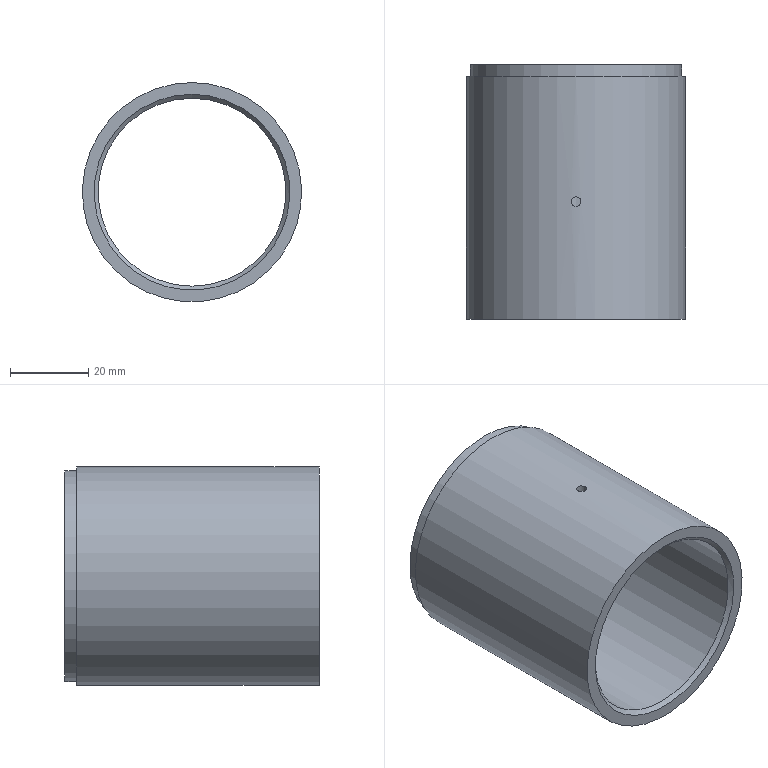Part | STEP file | JBJ-P-1016-01 | 1 solid | 8 faces | box 56 x 65 x 56 mm | volume 41860 mm3 | cylinder 4 | plane 3 | cone 1 | commonest cylinder face diameters 2.5 x1 48 x1 54 x1 56 x1
STEP:
#1=CARTESIAN_POINT('',(0.,62.,27.));
#2=VERTEX_POINT('',#1);
#3=CARTESIAN_POINT('',(0.,62.,0.));
#4=DIRECTION('',(0.,1.,0.));
#5=DIRECTION('',(0.,0.,1.));
#6=AXIS2_PLACEMENT_3D('',#3,#4,#5);
#7=CIRCLE('',#6,27.);
#8=EDGE_CURVE('',#2,#2,#7,.T.);
#9=ORIENTED_EDGE('',*,*,#8,.F.);
#10=EDGE_LOOP('',(#9));
#11=FACE_BOUND('',#10,.T.);
#12=CARTESIAN_POINT('',(0.,62.,28.));
#13=VERTEX_POINT('',#12);
#14=CARTESIAN_POINT('',(0.,62.,0.));
#15=DIRECTION('',(0.,1.,0.));
#16=DIRECTION('',(0.,0.,1.));
#17=AXIS2_PLACEMENT_3D('',#14,#15,#16);
#18=CIRCLE('',#17,28.);
#19=EDGE_CURVE('',#13,#13,#18,.T.);
#20=ORIENTED_EDGE('',*,*,#19,.T.);
#21=EDGE_LOOP('',(#20));
#22=FACE_OUTER_BOUND('',#21,.T.);
#23=CARTESIAN_POINT('',(0.,62.,0.));
#24=DIRECTION('',(0.,1.,0.));
#25=DIRECTION('',(0.,0.,1.));
#26=AXIS2_PLACEMENT_3D('',#23,#24,#25);
#27=PLANE('',#26);
#28=ADVANCED_FACE('',(#11,#22),#27,.T.);
#29=CARTESIAN_POINT('',(0.,0.,25.));
#30=VERTEX_POINT('',#29);
#31=CARTESIAN_POINT('',(0.,0.,0.));
#32=DIRECTION('',(0.,1.,0.));
#33=DIRECTION('',(0.,0.,1.));
#34=AXIS2_PLACEMENT_3D('',#31,#32,#33);
#35=CIRCLE('',#34,25.);
#36=EDGE_CURVE('',#30,#30,#35,.T.);
#37=ORIENTED_EDGE('',*,*,#36,.T.);
#38=EDGE_LOOP('',(#37));
#39=FACE_BOUND('',#38,.T.);
#40=CARTESIAN_POINT('',(0.,0.,28.));
#41=VERTEX_POINT('',#40);
#42=CARTESIAN_POINT('',(0.,0.,0.));
#43=DIRECTION('',(0.,1.,0.));
#44=DIRECTION('',(0.,0.,1.));
#45=AXIS2_PLACEMENT_3D('',#42,#43,#44);
#46=CIRCLE('',#45,28.);
#47=EDGE_CURVE('',#41,#41,#46,.T.);
#48=ORIENTED_EDGE('',*,*,#47,.F.);
#49=EDGE_LOOP('',(#48));
#50=FACE_OUTER_BOUND('',#49,.T.);
#51=CARTESIAN_POINT('',(0.,0.,0.));
#52=DIRECTION('',(0.,1.,0.));
#53=DIRECTION('',(0.,0.,1.));
#54=AXIS2_PLACEMENT_3D('',#51,#52,#53);
#55=PLANE('',#54);
#56=ADVANCED_FACE('',(#39,#50),#55,.F.);
#57=CARTESIAN_POINT('',(0.,28.75,28.));
#58=VERTEX_POINT('',#57);
#59=CARTESIAN_POINT('',(0.,28.75,28.));
#60=CARTESIAN_POINT('',(-0.1652,28.75,28.));
#61=CARTESIAN_POINT('',(-0.3273,28.783,27.998));
#62=CARTESIAN_POINT('',(-0.63,28.908,27.993));
#63=CARTESIAN_POINT('',(-0.7687,29.001,27.99));
#64=CARTESIAN_POINT('',(-0.9993,29.232,27.982));
#65=CARTESIAN_POINT('',(-1.092,29.371,27.979));
#66=CARTESIAN_POINT('',(-1.217,29.672,27.974));
#67=CARTESIAN_POINT('',(-1.25,29.836,27.972));
#68=CARTESIAN_POINT('',(-1.25,30.162,27.972));
#69=CARTESIAN_POINT('',(-1.218,30.326,27.974));
#70=CARTESIAN_POINT('',(-1.093,30.629,27.979));
#71=CARTESIAN_POINT('',(-1.001,30.767,27.982));
#72=CARTESIAN_POINT('',(-0.7677,31.,27.99));
#73=CARTESIAN_POINT('',(-0.6301,31.092,27.993));
#74=CARTESIAN_POINT('',(-0.4029,31.186,27.997));
#75=CARTESIAN_POINT('',(-0.325,31.21,27.998));
#76=CARTESIAN_POINT('',(-0.1649,31.242,28.));
#77=CARTESIAN_POINT('',(-0.08202,31.25,28.));
#78=CARTESIAN_POINT('',(0.1627,31.25,28.));
#79=CARTESIAN_POINT('',(0.3272,31.217,27.998));
#80=CARTESIAN_POINT('',(0.6281,31.093,27.993));
#81=CARTESIAN_POINT('',(0.7677,31.,27.99));
#82=CARTESIAN_POINT('',(0.9984,30.77,27.982));
#83=CARTESIAN_POINT('',(1.091,30.631,27.979));
#84=CARTESIAN_POINT('',(1.217,30.329,27.974));
#85=CARTESIAN_POINT('',(1.25,30.166,27.972));
#86=CARTESIAN_POINT('',(1.25,29.836,27.972));
#87=CARTESIAN_POINT('',(1.218,29.674,27.974));
#88=CARTESIAN_POINT('',(1.124,29.447,27.977));
#89=CARTESIAN_POINT('',(1.085,29.375,27.979));
#90=CARTESIAN_POINT('',(0.995,29.239,27.982));
#91=CARTESIAN_POINT('',(0.9422,29.175,27.984));
#92=CARTESIAN_POINT('',(0.7693,29.001,27.99));
#93=CARTESIAN_POINT('',(0.63,28.908,27.993));
#94=CARTESIAN_POINT('',(0.3293,28.783,27.998));
#95=CARTESIAN_POINT('',(0.1652,28.75,28.));
#96=CARTESIAN_POINT('',(0.,28.75,28.));
#97=B_SPLINE_CURVE_WITH_KNOTS('',3,(#59,#60,#61,#62,#63,#64,#65,#66,#67,#68,#69,#70,#71,#72,#73,#74,#75,#76,#77,#78,#79,#80,#81,#82,#83,#84,#85,#86,#87,#88,#89,#90,#91,#92,#93,#94,#95,#96),.UNSPECIFIED.,.T.,.F.,(4,2,2,2,2,2,2,2,2,2,2,2,2,2,2,2,2,2,4),(0.,0.0004885,0.000977,0.001466,0.001954,0.002443,0.002931,0.00342,0.003664,0.003908,0.004397,0.004885,0.005374,0.005862,0.006351,0.006595,0.006839,0.007328,0.007816),.UNSPECIFIED.);
#98=EDGE_CURVE('',#58,#58,#97,.T.);
#99=ORIENTED_EDGE('',*,*,#98,.T.);
#100=EDGE_LOOP('',(#99));
#101=FACE_BOUND('',#100,.T.);
#102=ORIENTED_EDGE('',*,*,#19,.F.);
#103=EDGE_LOOP('',(#102));
#104=FACE_OUTER_BOUND('',#103,.T.);
#105=ORIENTED_EDGE('',*,*,#47,.T.);
#106=EDGE_LOOP('',(#105));
#107=FACE_OUTER_BOUND('',#106,.T.);
#108=CARTESIAN_POINT('',(0.,62.,0.));
#109=DIRECTION('',(0.,-1.,0.));
#110=DIRECTION('',(0.,0.,-1.));
#111=AXIS2_PLACEMENT_3D('',#108,#109,#110);
#112=CYLINDRICAL_SURFACE('',#111,28.);
#113=ADVANCED_FACE('',(#101,#104,#107),#112,.T.);
#114=CARTESIAN_POINT('',(0.,1.,24.));
#115=VERTEX_POINT('',#114);
#116=CARTESIAN_POINT('',(0.,1.,0.));
#117=DIRECTION('',(0.,-1.,0.));
#118=DIRECTION('',(0.,0.,1.));
#119=AXIS2_PLACEMENT_3D('',#116,#117,#118);
#120=CIRCLE('',#119,24.);
#121=EDGE_CURVE('',#115,#115,#120,.T.);
#122=ORIENTED_EDGE('',*,*,#121,.T.);
#123=EDGE_LOOP('',(#122));
#124=FACE_OUTER_BOUND('',#123,.T.);
#125=CARTESIAN_POINT('',(-1.25,30.,23.967));
#126=VERTEX_POINT('',#125);
#127=CARTESIAN_POINT('',(-1.25,30.,23.967));
#128=CARTESIAN_POINT('',(-1.25,30.165,23.967));
#129=CARTESIAN_POINT('',(-1.217,30.327,23.969));
#130=CARTESIAN_POINT('',(-1.092,30.63,23.975));
#131=CARTESIAN_POINT('',(-0.9991,30.769,23.979));
#132=CARTESIAN_POINT('',(-0.7685,30.999,23.988));
#133=CARTESIAN_POINT('',(-0.6291,31.092,23.992));
#134=CARTESIAN_POINT('',(-0.3282,31.217,23.998));
#135=CARTESIAN_POINT('',(-0.1637,31.25,24.));
#136=CARTESIAN_POINT('',(0.1624,31.25,24.));
#137=CARTESIAN_POINT('',(0.3263,31.218,23.998));
#138=CARTESIAN_POINT('',(0.629,31.093,23.992));
#139=CARTESIAN_POINT('',(0.7667,31.001,23.988));
#140=CARTESIAN_POINT('',(1.,30.768,23.979));
#141=CARTESIAN_POINT('',(1.092,30.63,23.975));
#142=CARTESIAN_POINT('',(1.186,30.403,23.971));
#143=CARTESIAN_POINT('',(1.21,30.325,23.969));
#144=CARTESIAN_POINT('',(1.242,30.165,23.968));
#145=CARTESIAN_POINT('',(1.25,30.082,23.967));
#146=CARTESIAN_POINT('',(1.25,29.837,23.967));
#147=CARTESIAN_POINT('',(1.217,29.673,23.969));
#148=CARTESIAN_POINT('',(1.093,29.372,23.975));
#149=CARTESIAN_POINT('',(0.9999,29.232,23.979));
#150=CARTESIAN_POINT('',(0.7696,29.002,23.988));
#151=CARTESIAN_POINT('',(0.6309,28.909,23.992));
#152=CARTESIAN_POINT('',(0.3286,28.783,23.998));
#153=CARTESIAN_POINT('',(0.1662,28.75,24.));
#154=CARTESIAN_POINT('',(-0.1637,28.75,24.));
#155=CARTESIAN_POINT('',(-0.326,28.782,23.998));
#156=CARTESIAN_POINT('',(-0.5534,28.876,23.994));
#157=CARTESIAN_POINT('',(-0.6252,28.915,23.992));
#158=CARTESIAN_POINT('',(-0.7611,29.005,23.988));
#159=CARTESIAN_POINT('',(-0.8255,29.058,23.986));
#160=CARTESIAN_POINT('',(-0.9986,29.231,23.979));
#161=CARTESIAN_POINT('',(-1.092,29.37,23.975));
#162=CARTESIAN_POINT('',(-1.217,29.671,23.969));
#163=CARTESIAN_POINT('',(-1.25,29.835,23.967));
#164=CARTESIAN_POINT('',(-1.25,30.,23.967));
#165=B_SPLINE_CURVE_WITH_KNOTS('',3,(#127,#128,#129,#130,#131,#132,#133,#134,#135,#136,#137,#138,#139,#140,#141,#142,#143,#144,#145,#146,#147,#148,#149,#150,#151,#152,#153,#154,#155,#156,#157,#158,#159,#160,#161,#162,#163,#164),.UNSPECIFIED.,.T.,.F.,(4,2,2,2,2,2,2,2,2,2,2,2,2,2,2,2,2,2,4),(0.,0.0004885,0.0009771,0.001466,0.001954,0.002443,0.002931,0.00342,0.003664,0.003908,0.004397,0.004885,0.005374,0.005862,0.006351,0.006595,0.00684,0.007328,0.007817),.UNSPECIFIED.);
#166=EDGE_CURVE('',#126,#126,#165,.T.);
#167=ORIENTED_EDGE('',*,*,#166,.F.);
#168=EDGE_LOOP('',(#167));
#169=FACE_BOUND('',#168,.T.);
#170=CARTESIAN_POINT('',(0.,65.,24.));
#171=VERTEX_POINT('',#170);
#172=CARTESIAN_POINT('',(0.,65.,0.));
#173=DIRECTION('',(0.,1.,0.));
#174=DIRECTION('',(0.,0.,1.));
#175=AXIS2_PLACEMENT_3D('',#172,#173,#174);
#176=CIRCLE('',#175,24.);
#177=EDGE_CURVE('',#171,#171,#176,.T.);
#178=ORIENTED_EDGE('',*,*,#177,.T.);
#179=EDGE_LOOP('',(#178));
#180=FACE_OUTER_BOUND('',#179,.T.);
#181=CARTESIAN_POINT('',(0.,62.,0.));
#182=DIRECTION('',(0.,-1.,0.));
#183=DIRECTION('',(0.,0.,-1.));
#184=AXIS2_PLACEMENT_3D('',#181,#182,#183);
#185=CYLINDRICAL_SURFACE('',#184,24.);
#186=ADVANCED_FACE('',(#124,#169,#180),#185,.F.);
#187=CARTESIAN_POINT('',(0.,65.,27.));
#188=VERTEX_POINT('',#187);
#189=CARTESIAN_POINT('',(0.,65.,0.));
#190=DIRECTION('',(0.,1.,0.));
#191=DIRECTION('',(0.,0.,1.));
#192=AXIS2_PLACEMENT_3D('',#189,#190,#191);
#193=CIRCLE('',#192,27.);
#194=EDGE_CURVE('',#188,#188,#193,.T.);
#195=ORIENTED_EDGE('',*,*,#194,.T.);
#196=EDGE_LOOP('',(#195));
#197=FACE_OUTER_BOUND('',#196,.T.);
#198=ORIENTED_EDGE('',*,*,#177,.F.);
#199=EDGE_LOOP('',(#198));
#200=FACE_BOUND('',#199,.T.);
#201=CARTESIAN_POINT('',(0.,65.,0.));
#202=DIRECTION('',(0.,1.,0.));
#203=DIRECTION('',(0.,0.,1.));
#204=AXIS2_PLACEMENT_3D('',#201,#202,#203);
#205=PLANE('',#204);
#206=ADVANCED_FACE('',(#197,#200),#205,.T.);
#207=ORIENTED_EDGE('',*,*,#194,.F.);
#208=EDGE_LOOP('',(#207));
#209=FACE_OUTER_BOUND('',#208,.T.);
#210=ORIENTED_EDGE('',*,*,#8,.T.);
#211=EDGE_LOOP('',(#210));
#212=FACE_OUTER_BOUND('',#211,.T.);
#213=CARTESIAN_POINT('',(0.,65.,0.));
#214=DIRECTION('',(0.,-1.,0.));
#215=DIRECTION('',(0.,0.,-1.));
#216=AXIS2_PLACEMENT_3D('',#213,#214,#215);
#217=CYLINDRICAL_SURFACE('',#216,27.);
#218=ADVANCED_FACE('',(#209,#212),#217,.T.);
#219=ORIENTED_EDGE('',*,*,#166,.T.);
#220=EDGE_LOOP('',(#219));
#221=FACE_OUTER_BOUND('',#220,.T.);
#222=ORIENTED_EDGE('',*,*,#98,.F.);
#223=EDGE_LOOP('',(#222));
#224=FACE_OUTER_BOUND('',#223,.T.);
#225=CARTESIAN_POINT('',(0.,30.,0.));
#226=DIRECTION('',(0.,0.,-1.));
#227=DIRECTION('',(-1.,0.,0.));
#228=AXIS2_PLACEMENT_3D('',#225,#226,#227);
#229=CYLINDRICAL_SURFACE('',#228,1.25);
#230=ADVANCED_FACE('',(#221,#224),#229,.F.);
#231=ORIENTED_EDGE('',*,*,#121,.F.);
#232=EDGE_LOOP('',(#231));
#233=FACE_BOUND('',#232,.T.);
#234=ORIENTED_EDGE('',*,*,#36,.F.);
#235=EDGE_LOOP('',(#234));
#236=FACE_OUTER_BOUND('',#235,.T.);
#237=CARTESIAN_POINT('',(0.,0.,0.));
#238=DIRECTION('',(0.,-1.,0.));
#239=DIRECTION('',(0.,0.,-1.));
#240=AXIS2_PLACEMENT_3D('',#237,#238,#239);
#241=CONICAL_SURFACE('',#240,25.,0.7854);
#242=ADVANCED_FACE('',(#233,#236),#241,.F.);
#243=CLOSED_SHELL('',(#28,#56,#113,#186,#206,#218,#230,#242));
#244=MANIFOLD_SOLID_BREP('',#243);
#245=CARTESIAN_POINT('',(0.,0.,0.));
#246=DIRECTION('',(0.,0.,1.));
#247=DIRECTION('',(1.,0.,0.));
#248=AXIS2_PLACEMENT_3D('',#245,#246,#247);
#249=(LENGTH_UNIT()NAMED_UNIT(*)SI_UNIT(.MILLI.,.METRE.));
#250=UNCERTAINTY_MEASURE_WITH_UNIT(LENGTH_MEASURE(0.00001),#249,'','');
#251=(NAMED_UNIT(*)PLANE_ANGLE_UNIT()SI_UNIT($,.RADIAN.));
#252=(NAMED_UNIT(*)SI_UNIT($,.STERADIAN.)SOLID_ANGLE_UNIT());
#253=(GEOMETRIC_REPRESENTATION_CONTEXT(3)GLOBAL_UNCERTAINTY_ASSIGNED_CONTEXT((#250))GLOBAL_UNIT_ASSIGNED_CONTEXT((#249,#251,#252))REPRESENTATION_CONTEXT('',''));
#254=ADVANCED_BREP_SHAPE_REPRESENTATION('',(#244,#248),#253);